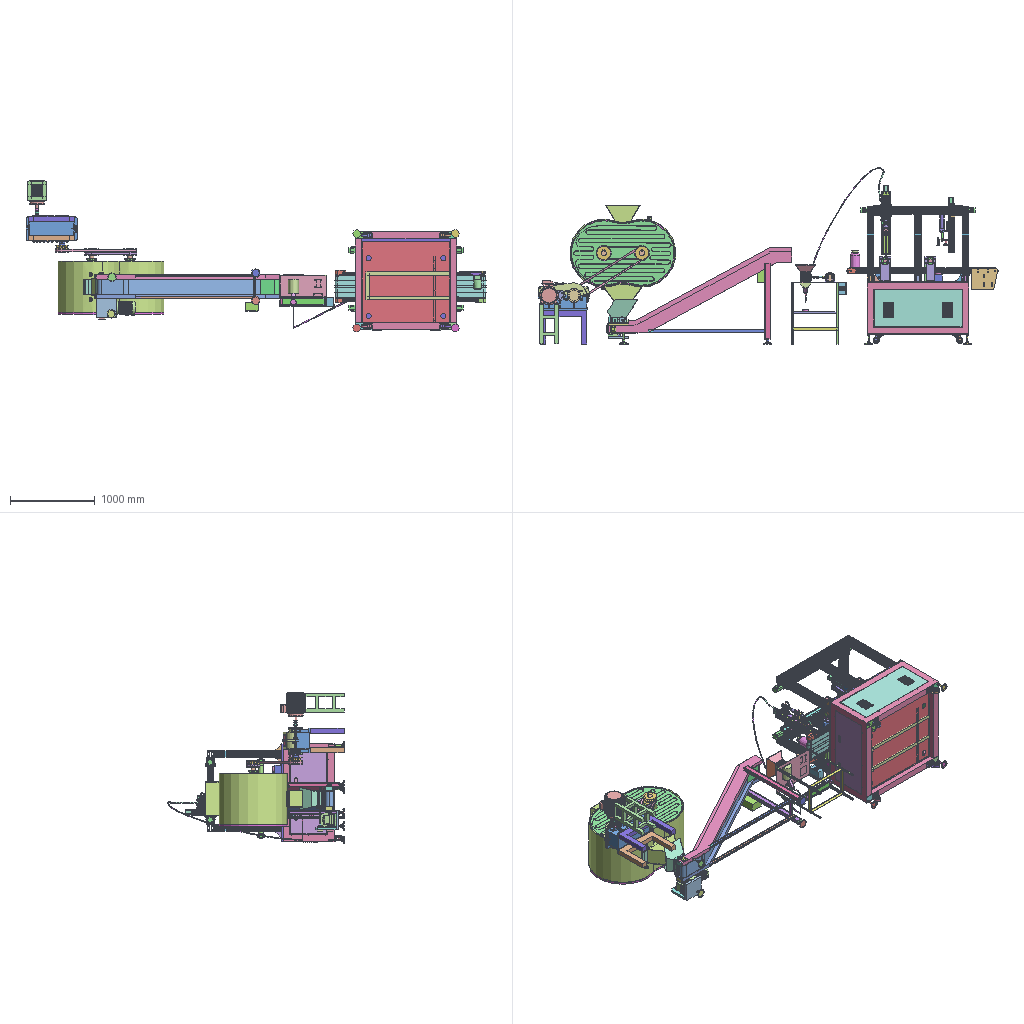Assembly | NX | 294 different items | 581 placed | box 5417 x 2077 x 1782 mm
Parts list (item | quantity | parent item | size | volume):
1 | x1 | in 70 | 2 x 18 x 18 mm | 395.448 mm3
2 | x1 | in 69 | 50 x 50 x 350 mm | 498728 mm3
3 | x1 | in 69 | 50 x 50 x 330 mm | 510150 mm3
4 | x1 | in 69 | 1780 x 70 x 255 mm | 4950684 mm3
5 | x1 | in 69 | 129.118 x 190 x 12 mm | 54428 mm3
6 | x1 | in 69 | 1050 x 535 x 330 mm | 11232000 mm3
7 | x2 | in 69 | 324 x 318 x 120 mm | 780087 mm3
8 | x2 | in 94 | 74.5 x 74 x 354 mm | 615079 mm3
9 | x1 | in 101 | 365 x 5 x 550 mm | 899488 mm3
10 | x1 | in 101 | 116 x 118 x 170 mm | 1317938 mm3
11 | x8 | in 63 | 14 x 14 x 12 mm | 1150 mm3
12 | x8 | in 94 | 14 x 14 x 12 mm | 1150 mm3
13 | x1 | in 70 | 603 x 172 x 290 mm | 5155522 mm3
14 | x20 | in 101 | 78.252 x 78.252 x 5 mm | 21007 mm3
15 | x20 | in 101 | 50 x 50 x 5 mm | 8518 mm3
16 | x1 | in 101 | 122 x 61 x 170 mm | 83012 mm3
17 | x1 | in 101 | 100 x 150 x 2 mm | 27600 mm3
18 | x2 | in 101 | 5 x 120 x 120 mm | 71829 mm3
19 | x2 | in 101 | 160 x 120 x 10 mm | 163934 mm3
20 | x1 | in 101 | 20 x 20 x 100 mm | 31416 mm3
21 | x2 | in 101 | 20 x 17.321 x 180 mm | 46765 mm3
22 | x1 | in 100 | 294 x 20 x 21 mm | 117693 mm3
23 | x2 | in 100 | 63 x 25 x 86 mm | 105613 mm3
24 | x2 | in 55 | 2 x 165 x 165 mm | 17394 mm3
25 | x2 | in 61 | 405 x 16 x 16 mm | 76382 mm3
26 | x2 | in 233 | 405 x 16 x 16 mm | 76382 mm3
27 | x2 | in 61 | 47 x 38 x 44 mm | 27725 mm3
28 | x2 | in 233 | 47 x 38 x 44 mm | 27725 mm3
29 | x1 | - | 23 x 26.558 x 246.5 mm | 74828 mm3
30 | x1 | - | 62 x 62 x 233 mm | 494308 mm3
31 | x2 | in 101 | 22 x 22 x 50 mm | 4852 mm3
32 | x1 | in 101 | 22 x 22 x 50 mm | 7499 mm3
33 | x20 | in 101 | 47.73 x 120 x 5 mm | 17127 mm3
34 | x1 | in 41 | 32 x 32 x 3.35 mm | 547.109 mm3
35 | x1 | - | 32 x 32 x 3.35 mm | 547.109 mm3
36 | x1 | in 41 | 104 x 47 x 100 mm | 229992 mm3
37 | x1 | - | 104 x 47 x 100 mm | 229992 mm3
38 | x1 | in 41 | 100 x 46 x 720 mm | 991013 mm3
39 | x1 | in 55 | 85 x 9.087 x 85 mm | 16353 mm3
40 | x1 | - | 100 x 46 x 560 mm | 769378 mm3
41 | x1 | in 95 | 120 x 94.5 x 821 mm | 2387862 mm3
42 | x1 | - | - | -
43 | x1 | in 41 | 100 x 69 x 8 mm | 19281 mm3
44 | x1 | - | 100 x 69 x 8 mm | 19281 mm3
45 | x1 | in 41 | 100 x 66 x 12 mm | 66555 mm3
46 | x1 | in 41 | 10 x 120 x 150 mm | 180000 mm3
47 | x1 | in 41 | 10 x 110 x 105 mm | 112434 mm3
48 | x1 | - | 10 x 110 x 105 mm | 112434 mm3
49 | x2 | in 63 | 40 x 120 x 74.319 mm | 278660 mm3
50 | x2 | in 94 | 40 x 120 x 74.319 mm | 278660 mm3
51 | x2 | in 41 | 8 x 26 x 26 mm | 2622 mm3
52 | x2 | - | 8 x 26 x 26 mm | 2622 mm3
53 | x4 | in 61 | 8 x 28 x 28 mm | 2885 mm3
54 | x4 | in 233 | 8 x 28 x 28 mm | 2885 mm3
55 | x1 | in 70 | 258.17 x 436.9 x 258.17 mm | 5108197 mm3
56 | x1 | in 101 | 20 x 40 x 20 mm | 3040 mm3
57 | x2 | in 61 | 8 x 28 x 28 mm | 2977 mm3
58 | x2 | in 233 | 8 x 28 x 28 mm | 2977 mm3
59 | x1 | in 41 | 8 x 26 x 26 mm | 2693 mm3
60 | x1 | - | 8 x 26 x 26 mm | 2693 mm3
61 | x1 | - | 110 x 95.023 x 1344 mm | 4565293 mm3
62 | x2 | in 63 | 74.5 x 74 x 354 mm | 615079 mm3
63 | x2 | - | 74.5 x 129 x 396.319 mm | 982754 mm3
64 | x8 | in 101 | 8 x 5.5 x 5.5 mm | 97.562 mm3
65 | x2 | in 70 | 16.097 x 16.1 x 2.6 mm | 277.756 mm3
66 | x2 | in 101 | 12 x 70.969 x 70.969 mm | 36930 mm3
67 | x2 | in 61 | 50 x 15 x 63 mm | 38157 mm3
68 | x2 | in 233 | 50 x 15 x 63 mm | 38157 mm3
69 | x1 | - | 1780 x 728 x 380 mm | 26797017 mm3
70 | x1 | in 85 | - | -
71 | x2 | in 90 | 1210 x 760 x 3.5 mm | 1542690 mm3
72 | x1 | - | 50 x 58 x 50 mm | 30230 mm3
73 | x1 | in 55 | 14 x 18 x 100 mm | 24227 mm3
74 | x1 | - | 30 x 93.15 x 30 mm | 27021 mm3
75 | x2 | in 61 | - | -
76 | x2 | in 233 | - | -
77 | x1 | - | 35 x 100 x 100 mm | 150000 mm3
78 | x1 | - | 92 x 117 x 105 mm | 132849 mm3
79 | x2 | - | 129 x 292 x 584 mm | 817102 mm3
80 | x1 | in 90 | 610 x 160 x 30 mm | 573090 mm3
81 | x1 | in 85 | 160 x 160 x 80 mm | 966511 mm3
82 | x2 | in 90 | 160 x 160 x 80 mm | 966511 mm3
83 | x1 | in 85 | - | -
84 | x1 | in 100 | 48.781 x 356.5 x 38.5 mm | 209713 mm3
85 | x1 | - | - | -
86 | x1 | in 55 | 165 x 30.6 x 165 mm | 204045 mm3
87 | x2 | in 90 | 120 x 120 x 10 mm | 107395 mm3
88 | x2 | in 90 | 120 x 120 x 10 mm | 87760 mm3
89 | x2 | in 90 | 591.212 x 581.908 x 770 mm | 2385468 mm3
90 | x1 | in 85 | 1280 x 1146 x 788 mm | 50655917 mm3
91 | x1 | in 95 | - | 96365724 mm3
92 | x8 | in 61 | 10 x 16 x 16 mm | 1700 mm3
93 | x8 | in 233 | 10 x 16 x 16 mm | 1700 mm3
94 | x2 | - | 74.5 x 129 x 396.319 mm | 982754 mm3
95 | x1 | - | - | 110218188 mm3
96 | x1 | - | 110 x 202 x 110 mm | 227376 mm3
97 | x1 | in 85 | 362.6 x 286.311 x 222.656 mm | 9083638 mm3
98 | x2 | in 203 | 120 x 120 x 2 mm | 11739 mm3
99 | x1 | in 90 | 959.982 x 659.964 x 30 mm | 993346 mm3
100 | x1 | in 95 | 112.8 x 138 x 491.298 mm | 1337292 mm3
101 | x1 | - | 377.735 x 640.424 x 932.038 mm | 5983886 mm3
102 | x1 | in 85 | 40 x 40 x 57.5 mm | 43840 mm3
103 | x1 | - | 100 x 66 x 12 mm | 66555 mm3
104 | x2 | in 61 | 35 x 35 x 8 mm | 4613 mm3
105 | x2 | in 233 | 35 x 35 x 8 mm | 4613 mm3
106 | x1 | in 41 | 60 x 70 x 60 mm | 117109 mm3
107 | x1 | - | 60 x 70 x 60 mm | 117109 mm3
108 | x1 | in 41 | 35 x 35 x 8 mm | 5240 mm3
109 | x1 | - | 35 x 35 x 8 mm | 5240 mm3
110 | x1 | in 180 | 48 x 887.916 x 72 mm | 888366 mm3
111 | x1 | in 180 | 24 x 62.191 x 60 mm | 81725 mm3
112 | x1 | in 203 | 80 x 26.5 x 80 mm | 32281 mm3
113 | x1 | in 180 | 24 x 36 x 60 mm | 51081 mm3
114 | x1 | in 180 | 270 x 276 x 360.692 mm | 479442 mm3
115 | x1 | in 180 | 268.32 x 36 x 24 mm | 55317 mm3
116 | x1 | in 180 | 180 x 90 x 90 mm | 1145111 mm3
117 | x1 | in 180 | 180 x 102 x 280.001 mm | 706349 mm3
118 | x1 | in 180 | 137.023 x 18 x 26.957 mm | 66486 mm3
119 | x1 | in 180 | 137.023 x 18 x 49.799 mm | 122824 mm3
120 | x1 | in 180 | 102 x 220.092 x 150 mm | 3361772 mm3
121 | x1 | in 180 | 18 x 21.457 x 240 mm | 48179 mm3
122 | x1 | in 180 | 24 x 75.39 x 75.33 mm | 52699 mm3
123 | x2 | in 70 | 16 x 18.475 x 46.4 mm | 4387 mm3
124 | x1 | in 203 | 14 x 45 x 10 mm | 5879 mm3
125 | x1 | in 180 | 24 x 75.378 x 75.347 mm | 52699 mm3
126 | x1 | in 180 | 100.8 x 136.08 x 100.8 mm | 135475 mm3
127 | x1 | in 180 | 30 x 27 x 27 mm | 9581 mm3
128 | x1 | in 180 | 180 x 945 x 1950 mm | 4768018 mm3
129 | x1 | in 180 | 15 x 60 x 60 mm | 52304 mm3
130 | x1 | in 180 | 15.665 x 95.15 x 95.15 mm | 40283 mm3
131 | x2 | in 203 | 80 x 80 x 18 mm | 45313 mm3
132 | x1 | in 180 | 100.8 x 136.08 x 100.8 mm | 135475 mm3
133 | x1 | in 180 | 156 x 17.318 x 18.649 mm | 12986 mm3
134 | x1 | in 180 | 100.8 x 136.08 x 100.8 mm | 135475 mm3
135 | x1 | in 180 | 156 x 21.463 x 12.735 mm | 12986 mm3
136 | x1 | in 180 | 180 x 28.797 x 45.12 mm | 16262 mm3
137 | x1 | in 180 | 15.665 x 95.16 x 95.16 mm | 40283 mm3
138 | x1 | in 180 | 100.8 x 136.08 x 100.8 mm | 135475 mm3
139 | x1 | in 203 | 214.08 x 214.08 x 50 mm | 1001272 mm3
140 | x1 | in 180 | 18 x 21.457 x 240 mm | 48179 mm3
141 | x1 | in 180 | 48 x 1000 x 2173 mm | 15101075 mm3
142 | x1 | in 180 | 48 x 1000 x 2173 mm | 15101075 mm3
143 | x1 | in 180 | 228 x 33 x 240 mm | 1805760 mm3
144 | x1 | in 180 | 24 x 240 x 120 mm | 683424 mm3
145 | x1 | in 180 | 15 x 60 x 60 mm | 51349 mm3
146 | x1 | in 180 | 48 x 6 x 72 mm | 20261 mm3
147 | x1 | in 180 | 48 x 6 x 72 mm | 20261 mm3
148 | x1 | in 180 | 15 x 60 x 60 mm | 51475 mm3
149 | x1 | in 180 | 210 x 198.012 x 456.821 mm | 7325207 mm3
150 | x1 | in 199 | 112 x 37.6 x 112 mm | 122481 mm3
151 | x1 | in 180 | 258 x 14.64 x 14.64 mm | 43430 mm3
152 | x1 | in 180 | 15 x 60 x 60 mm | 52304 mm3
153 | x1 | in 180 | 180 x 18 x 3.6 mm | 11664 mm3
154 | x1 | in 180 | 156 x 21.213 x 13.442 mm | 12986 mm3
155 | x1 | in 180 | 156 x 8.225 x 21.556 mm | 12986 mm3
156 | x1 | in 180 | 258 x 14.64 x 14.64 mm | 43430 mm3
157 | x1 | in 180 | 15 x 60 x 60 mm | 52304 mm3
158 | x1 | in 180 | 156 x 9.133 x 21.7 mm | 12986 mm3
159 | x1 | in 180 | 54.267 x 95.886 x 18 mm | 92346 mm3
160 | x1 | in 180 | 156 x 20.879 x 9.622 mm | 12986 mm3
161 | x2 | in 199 | 72 x 72 x 17 mm | 35548 mm3
162 | x1 | in 180 | 15 x 60 x 60 mm | 52304 mm3
163 | x1 | in 180 | 156 x 20.992 x 8.474 mm | 12986 mm3
164 | x1 | in 180 | 54.267 x 95.886 x 18 mm | 92346 mm3
165 | x1 | in 180 | 156 x 15.189 x 19.275 mm | 12986 mm3
166 | x1 | in 180 | 48 x 887.916 x 72 mm | 888366 mm3
167 | x1 | in 180 | 156 x 16.712 x 19.269 mm | 12986 mm3
168 | x1 | in 180 | 156 x 14.259 x 19.552 mm | 12986 mm3
169 | x1 | in 180 | 252 x 42 x 42 mm | 239583 mm3
170 | x1 | in 180 | 252 x 42 x 42 mm | 239583 mm3
171 | x1 | in 180 | 24 x 36 x 1349 mm | 278141 mm3
172 | x1 | in 70 | 11.253 x 40.001 x 11.253 mm | 3063 mm3
173 | x1 | in 180 | 24 x 9.093 x 8.534 mm | 1037 mm3
174 | x1 | in 180 | 24 x 9.359 x 9.297 mm | 1037 mm3
175 | x1 | in 180 | 24 x 36 x 60 mm | 51081 mm3
176 | x1 | in 180 | 24 x 9.359 x 9.297 mm | 1037 mm3
177 | x1 | in 180 | 24 x 9.093 x 8.534 mm | 1037 mm3
178 | x1 | in 180 | 24 x 62.191 x 60 mm | 81725 mm3
179 | x1 | in 180 | 24 x 36 x 1349 mm | 278141 mm3
180 | x1 | - | 593.919 x 1135 x 2179 mm | 55419513 mm3
181 | x1 | - | 120 x 11.2 x 24.73 mm | 29940 mm3
182 | x1 | in 100 | 6 x 6 x 40 mm | 952.137 mm3
183 | x2 | in 70 | 18.475 x 16 x 9.5 mm | 1522 mm3
184 | x1 | in 100 | 459.645 x 60 x 17 mm | 444065 mm3
185 | x1 | in 100 | 49.6 x 41.3 x 40 mm | 1923 mm3
186 | x1 | in 100 | 67 x 50 x 30 mm | 41805 mm3
187 | x1 | in 100 | 12 x 12 x 46 mm | 4911 mm3
188 | x1 | in 100 | 18 x 18 x 3.5 mm | 714.091 mm3
189 | x1 | in 100 | 91 x 31 x 11 mm | 24094 mm3
190 | x1 | in 100 | 79.5 x 69 x 17 mm | 69323 mm3
191 | x1 | in 100 | 72 x 72 x 15 mm | 58991 mm3
192 | x1 | in 100 | 12 x 12 x 13 mm | 1303 mm3
193 | x1 | in 100 | 21 x 21 x 3.5 mm | 1036 mm3
194 | x2 | in 199 | 112 x 112 x 2 mm | 10734 mm3
195 | x1 | in 100 | 72 x 94 x 14 mm | 74402 mm3
196 | x1 | in 100 | 72 x 94 x 14 mm | 72983 mm3
197 | x1 | - | 106.8 x 119.1 x 80.79 mm | 246955 mm3
198 | x1 | in 199 | 112 x 37.6 x 112 mm | 108254 mm3
199 | x1 | in 70 | 112 x 366.9 x 112 mm | 770661 mm3
200 | x4 | in 70 | 11.547 x 10 x 24 mm | 859.994 mm3
201 | x1 | in 199 | 44 x 7.719 x 44 mm | 5537 mm3
202 | x2 | in 203 | 120 x 36.6 x 120 mm | 140285 mm3
203 | x1 | in 70 | 214.08 x 317.8 x 214.08 mm | 2085150 mm3
204 | x1 | in 55 | 20 x 70 x 14 mm | 18398 mm3
205 | x1 | in 55 | 165 x 30.6 x 165 mm | 264298 mm3
206 | x8 | in 70 | 21 x 24.249 x 108.8 mm | 18047 mm3
207 | x2 | in 61 | 166.5 x 75 x 60 mm | 436782 mm3
208 | x2 | in 233 | 166.5 x 75 x 60 mm | 436782 mm3
209 | x3 | in 95 | 800 x 80 x 80 mm | 1853836 mm3
210 | x3 | - | 800 x 80 x 80 mm | 1853836 mm3
211 | x1 | - | 585 x 80 x 80 mm | 1355618 mm3
212 | x2 | - | 1200 x 80 x 80 mm | 2780754 mm3
213 | x1 | in 70 | 603 x 149 x 284 mm | 3323600 mm3
214 | x1 | in 55 | 125 x 26.5 x 125 mm | 65845 mm3
215 | x1 | in 55 | 258.17 x 258.17 x 78 mm | 2559189 mm3
216 | x1 | in 55 | 125 x 15 x 125 mm | 51673 mm3
217 | x1 | in 203 | 70 x 14 x 10 mm | 9379 mm3
218 | x1 | in 203 | 80 x 26.5 x 80 mm | 32281 mm3
219 | x1 | in 203 | 83.83 x 83.83 x 81 mm | 243039 mm3
220 | x2 | in 199 | 72 x 15 x 72 mm | 19220 mm3
221 | x8 | in 70 | 22.096 x 22.1 x 3.6 mm | 729.48 mm3
222 | x1 | in 41 | 57 x 86 x 57 mm | 190967 mm3
223 | x1 | - | 57 x 86 x 57 mm | 190967 mm3
224 | x1 | in 70 | 18.475 x 16 x 36.4 mm | 3611 mm3
225 | x8 | in 70 | 24.249 x 21 x 13.9 mm | 3616 mm3
226 | x1 | in 69 | 90 x 90 x 193 mm | 1102309 mm3
227 | x1 | in 70 | 2 x 180 x 140 mm | 17112 mm3
228 | x1 | in 70 | 4 x 180 x 140 mm | 99996 mm3
229 | x1 | in 70 | 25 x 35 x 25 mm | 6094 mm3
230 | x4 | in 41 | 15 x 15 x 7 mm | 837.711 mm3
231 | x3 | - | 15 x 15 x 7 mm | 837.711 mm3
232 | x1 | - | 15 x 15 x 7 mm | 837.711 mm3
233 | x1 | in 95 | 110 x 95 x 1344 mm | 4565293 mm3
234 | x1 | in 61 | 95 x 64 x 1045 mm | 1787875 mm3
235 | x1 | in 233 | 95 x 64 x 1045 mm | 1787875 mm3
236 | x2 | in 61 | 60 x 88 x 77.5 mm | 126887 mm3
237 | x2 | in 233 | 60 x 88 x 77.5 mm | 126887 mm3
238 | x1 | - | 525 x 16 x 16 mm | 99560 mm3
239 | x2 | in 61 | 95 x 87 x 8 mm | 29353 mm3
240 | x2 | in 233 | 95 x 87 x 8 mm | 29353 mm3
241 | x2 | in 61 | 110 x 61.5 x 95 mm | 250471 mm3
242 | x2 | in 233 | 110 x 61.5 x 95 mm | 250471 mm3
243 | x1 | in 61 | 82 x 11 x 1061 mm | 230950 mm3
244 | x1 | in 233 | 82 x 11 x 1061 mm | 230950 mm3
245 | x1 | in 101 | 70 x 40 x 70 mm | 34909 mm3
246 | x1 | in 101 | 538 x 2 x 97 mm | 104372 mm3
247 | x2 | in 101 | 100 x 22 x 22 mm | 8400 mm3
248 | x2 | in 101 | 538 x 20 x 20 mm | 59718 mm3
249 | x4 | in 101 | 10 x 42 x 42 mm | 11256 mm3
250 | x1 | in 101 | 100 x 150 x 80 mm | 99552 mm3
251 | x1 | in 101 | 40 x 67.338 x 154.471 mm | 46471 mm3
252 | x1 | in 41 | 705 x 16 x 16 mm | 135751 mm3
253 | x2 | in 8 | 74.5 x 74 x 314 mm | 475496 mm3
254 | x2 | in 62 | 74.5 x 74 x 314 mm | 475496 mm3
255 | x1 | in 41 | 31.996 x 13.3 x 32 mm | 8366 mm3
256 | x1 | - | 31.996 x 13.3 x 32 mm | 8366 mm3
257 | x1 | in 41 | 31.996 x 13.3 x 32 mm | 8704 mm3
258 | x1 | - | 31.996 x 13.3 x 32 mm | 8704 mm3
259 | x1 | in 100 | 14 x 27.5 x 16 mm | 2157 mm3
260 | x2 | in 69 | 60 x 40 x 1600 mm | 2047255 mm3
261 | x1 | - | 15 x 12.5 x 300 mm | 47224 mm3
262 | x4 | in 61 | 560 x 12.5 x 15 mm | 104651 mm3
263 | x4 | in 233 | 560 x 12.5 x 15 mm | 104651 mm3
264 | x1 | in 41 | 15 x 12.5 x 610 mm | 97842 mm3
265 | x4 | in 61 | 56.8 x 19.5 x 34 mm | 29007 mm3
266 | x4 | in 233 | 56.8 x 19.5 x 34 mm | 29007 mm3
267 | x1 | in 41 | 34 x 19.5 x 57.8 mm | 30498 mm3
268 | x1 | - | 34 x 19.5 x 57.8 mm | 30498 mm3
269 | x1 | in 70 | 20.002 x 116.72 x 20.002 mm | 7452 mm3
270 | x2 | in 63 | 74 x 129 x 12 mm | 84307 mm3
271 | x2 | in 94 | 74 x 129 x 12 mm | 84307 mm3
272 | x4 | in 90 | 72 x 72 x 12 mm | 17105 mm3
273 | x2 | in 55 | 125 x 125 x 24 mm | 136380 mm3
274 | x18 | in 90 | 16 x 18.475 x 26.4 mm | 2900 mm3
275 | x12 | in 55 | 15.011 x 13 x 30.3 mm | 1931 mm3
276 | x12 | in 199 | 15.011 x 13 x 30.3 mm | 1931 mm3
277 | x12 | in 203 | 15.011 x 13 x 30.3 mm | 1931 mm3
278 | x18 | in 90 | 18 x 18 x 1.6 mm | 268.606 mm3
279 | x1 | - | 79 x 6 x 572 mm | 116838 mm3
280 | x1 | in 41 | 79 x 6 x 732 mm | 149566 mm3
281 | x1 | in 101 | 107 x 103 x 99.996 mm | 380295 mm3
282 | x2 | in 8 | 60 x 60 x 300 mm | 139937 mm3
283 | x2 | in 62 | 60 x 60 x 300 mm | 139937 mm3
284 | x1 | in 70 | 18 x 20 x 18 mm | 2389 mm3
285 | x2 | in 101 | 285.47 x 100 x 2 mm | 45085 mm3
286 | x2 | in 101 | 235.47 x 100 x 2 mm | 34997 mm3
287 | x1 | in 41 | 48 x 40 x 57 mm | 32709 mm3
288 | x1 | - | 48 x 40 x 57 mm | 32709 mm3
289 | x4 | in 101 | 20 x 724.234 x 20 mm | 147744 mm3
290 | x4 | in 69 | 30 x 30 x 260 mm | 183783 mm3
291 | x2 | in 69 | 120 x 60 x 50 mm | 252472 mm3
292 | x1 | in 69 | 120 x 60 x 50 mm | 271153 mm3
293 | x1 | in 69 | 313.118 x 250 x 15 mm | 1008735 mm3
294 | x1 | in 69 | 120 x 120 x 35 mm | 274066 mm3
Mates (type | each side: item.copy, entity, surface, feature):
Touch | 71.1 | assembly face